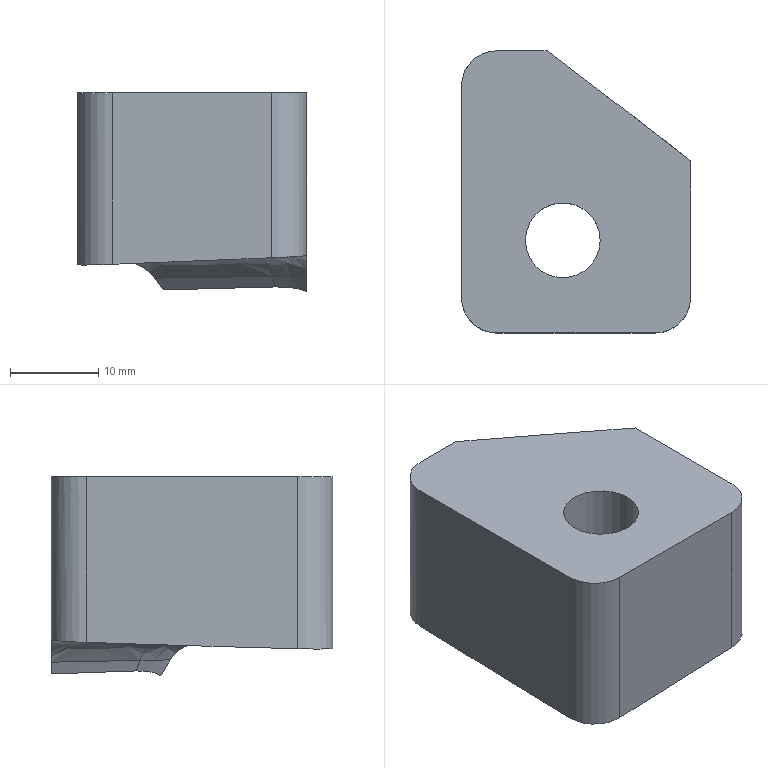Part | STEP file | gslz 2016.10.28-10_id1218_x_t | 1 solid | 18 faces | box 26 x 32 x 22.581 mm | volume 11602 mm3 | plane 6 | spline 6 | cylinder 5 | other 1 | commonest cylinder face diameters 8 x3 8.5 x1 14 x1